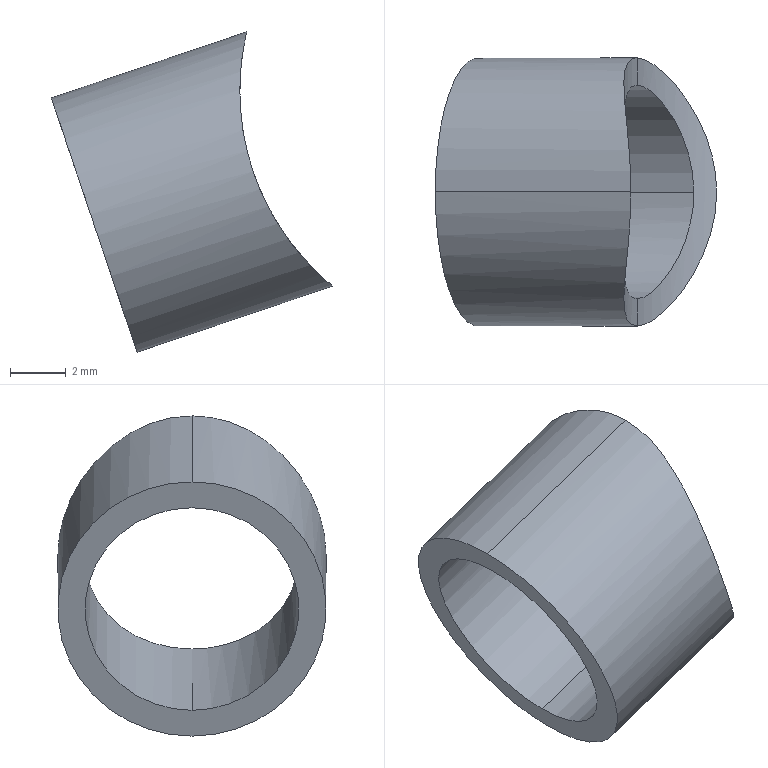Part | STEP file | 2026.6.15-Main Assembly图.sldasm-Part-265 | 1 solid | 7 faces | box 10.07 x 9.6 x 11.459 mm | volume 173.019 mm3 | cylinder 6 | plane 1 | commonest cylinder face diameters 7.65 x2 9.6 x2 18 x2
STEP:
#1=CARTESIAN_POINT('',(-1469.975,1419.464,3250.583));
#2=VERTEX_POINT('',#1);
#3=CARTESIAN_POINT('',(-1470.196,1424.264,3255.574));
#4=VERTEX_POINT('',#3);
#5=CARTESIAN_POINT('',(-1469.975,1419.464,3250.583));
#6=CARTESIAN_POINT('',(-1470.026,1419.464,3250.735));
#7=CARTESIAN_POINT('',(-1470.074,1419.472,3250.89));
#8=CARTESIAN_POINT('',(-1470.16,1419.505,3251.198));
#9=CARTESIAN_POINT('',(-1470.198,1419.529,3251.351));
#10=CARTESIAN_POINT('',(-1470.266,1419.592,3251.656));
#11=CARTESIAN_POINT('',(-1470.296,1419.631,3251.808));
#12=CARTESIAN_POINT('',(-1470.347,1419.724,3252.111));
#13=CARTESIAN_POINT('',(-1470.369,1419.779,3252.262));
#14=CARTESIAN_POINT('',(-1470.421,1419.963,3252.705));
#15=CARTESIAN_POINT('',(-1470.439,1420.111,3252.987));
#16=CARTESIAN_POINT('',(-1470.451,1420.459,3253.527));
#17=CARTESIAN_POINT('',(-1470.445,1420.658,3253.783));
#18=CARTESIAN_POINT('',(-1470.416,1421.092,3254.25));
#19=CARTESIAN_POINT('',(-1470.394,1421.33,3254.464));
#20=CARTESIAN_POINT('',(-1470.343,1421.847,3254.848));
#21=CARTESIAN_POINT('',(-1470.314,1422.118,3255.012));
#22=CARTESIAN_POINT('',(-1470.276,1422.548,3255.216));
#23=CARTESIAN_POINT('',(-1470.263,1422.695,3255.276));
#24=CARTESIAN_POINT('',(-1470.241,1422.996,3255.382));
#25=CARTESIAN_POINT('',(-1470.231,1423.152,3255.428));
#26=CARTESIAN_POINT('',(-1470.206,1423.622,3255.537));
#27=CARTESIAN_POINT('',(-1470.196,1423.94,3255.574));
#28=CARTESIAN_POINT('',(-1470.196,1424.264,3255.574));
#29=B_SPLINE_CURVE_WITH_KNOTS('',3,(#5,#6,#7,#8,#9,#10,#11,#12,#13,#14,#15,#16,#17,#18,#19,#20,#21,#22,#23,#24,#25,#26,#27,#28),.UNSPECIFIED.,.F.,.F.,(4,2,2,2,2,2,2,2,2,2,2,4),(0.007657,0.008135,0.008612,0.00909,0.009568,0.01052,0.01148,0.01243,0.01339,0.01387,0.01434,0.0153),.UNSPECIFIED.);
#30=EDGE_CURVE('',#2,#4,#29,.T.);
#31=ORIENTED_EDGE('',*,*,#30,.F.);
#32=CARTESIAN_POINT('',(-1469.975,1420.439,3250.583));
#33=VERTEX_POINT('',#32);
#34=CARTESIAN_POINT('',(-1469.975,1412.264,3250.583));
#35=DIRECTION('',(0.,1.,0.));
#36=VECTOR('',#35,1000.);
#37=LINE('',#34,#36);
#38=EDGE_CURVE('',#2,#33,#37,.T.);
#39=ORIENTED_EDGE('',*,*,#38,.T.);
#40=CARTESIAN_POINT('',(-1470.39,1424.264,3254.48));
#41=VERTEX_POINT('',#40);
#42=CARTESIAN_POINT('',(-1470.39,1424.264,3254.48));
#43=CARTESIAN_POINT('',(-1470.39,1424.008,3254.48));
#44=CARTESIAN_POINT('',(-1470.393,1423.757,3254.452));
#45=CARTESIAN_POINT('',(-1470.405,1423.264,3254.343));
#46=CARTESIAN_POINT('',(-1470.413,1423.02,3254.262));
#47=CARTESIAN_POINT('',(-1470.429,1422.558,3254.052));
#48=CARTESIAN_POINT('',(-1470.437,1422.34,3253.925));
#49=CARTESIAN_POINT('',(-1470.447,1421.926,3253.629));
#50=CARTESIAN_POINT('',(-1470.449,1421.733,3253.461));
#51=CARTESIAN_POINT('',(-1470.442,1421.385,3253.095));
#52=CARTESIAN_POINT('',(-1470.432,1421.227,3252.896));
#53=CARTESIAN_POINT('',(-1470.395,1420.948,3252.47));
#54=CARTESIAN_POINT('',(-1470.368,1420.831,3252.248));
#55=CARTESIAN_POINT('',(-1470.294,1420.639,3251.788));
#56=CARTESIAN_POINT('',(-1470.245,1420.564,3251.547));
#57=CARTESIAN_POINT('',(-1470.126,1420.464,3251.064));
#58=CARTESIAN_POINT('',(-1470.056,1420.439,3250.823));
#59=CARTESIAN_POINT('',(-1469.975,1420.439,3250.583));
#60=B_SPLINE_CURVE_WITH_KNOTS('',3,(#42,#43,#44,#45,#46,#47,#48,#49,#50,#51,#52,#53,#54,#55,#56,#57,#58,#59),.UNSPECIFIED.,.F.,.F.,(4,2,2,2,2,2,2,2,4),(0.,0.0007567,0.001513,0.00227,0.003027,0.003784,0.00454,0.005297,0.006054),.UNSPECIFIED.);
#61=EDGE_CURVE('',#41,#33,#60,.T.);
#62=ORIENTED_EDGE('',*,*,#61,.F.);
#63=CARTESIAN_POINT('',(-1469.975,1428.089,3250.583));
#64=VERTEX_POINT('',#63);
#65=CARTESIAN_POINT('',(-1469.975,1428.089,3250.583));
#66=CARTESIAN_POINT('',(-1470.055,1428.089,3250.822));
#67=CARTESIAN_POINT('',(-1470.127,1428.064,3251.069));
#68=CARTESIAN_POINT('',(-1470.245,1427.964,3251.549));
#69=CARTESIAN_POINT('',(-1470.293,1427.891,3251.787));
#70=CARTESIAN_POINT('',(-1470.369,1427.696,3252.253));
#71=CARTESIAN_POINT('',(-1470.396,1427.578,3252.474));
#72=CARTESIAN_POINT('',(-1470.432,1427.302,3252.896));
#73=CARTESIAN_POINT('',(-1470.442,1427.142,3253.098));
#74=CARTESIAN_POINT('',(-1470.449,1426.793,3253.463));
#75=CARTESIAN_POINT('',(-1470.447,1426.603,3253.629));
#76=CARTESIAN_POINT('',(-1470.437,1426.19,3253.925));
#77=CARTESIAN_POINT('',(-1470.429,1425.969,3254.053));
#78=CARTESIAN_POINT('',(-1470.413,1425.511,3254.261));
#79=CARTESIAN_POINT('',(-1470.405,1425.272,3254.341));
#80=CARTESIAN_POINT('',(-1470.393,1424.774,3254.452));
#81=CARTESIAN_POINT('',(-1470.39,1424.52,3254.48));
#82=CARTESIAN_POINT('',(-1470.39,1424.264,3254.48));
#83=B_SPLINE_CURVE_WITH_KNOTS('',3,(#65,#66,#67,#68,#69,#70,#71,#72,#73,#74,#75,#76,#77,#78,#79,#80,#81,#82),.UNSPECIFIED.,.F.,.F.,(4,2,2,2,2,2,2,2,4),(0.006054,0.006809,0.007565,0.00832,0.009076,0.009831,0.01059,0.01134,0.0121),.UNSPECIFIED.);
#84=EDGE_CURVE('',#64,#41,#83,.T.);
#85=ORIENTED_EDGE('',*,*,#84,.F.);
#86=CARTESIAN_POINT('',(-1469.975,1429.064,3250.583));
#87=VERTEX_POINT('',#86);
#88=CARTESIAN_POINT('',(-1469.975,1412.264,3250.583));
#89=DIRECTION('',(0.,1.,0.));
#90=VECTOR('',#89,1000.);
#91=LINE('',#88,#90);
#92=EDGE_CURVE('',#64,#87,#91,.T.);
#93=ORIENTED_EDGE('',*,*,#92,.T.);
#94=CARTESIAN_POINT('',(-1470.196,1424.264,3255.574));
#95=CARTESIAN_POINT('',(-1470.196,1424.589,3255.574));
#96=CARTESIAN_POINT('',(-1470.206,1424.906,3255.537));
#97=CARTESIAN_POINT('',(-1470.238,1425.528,3255.393));
#98=CARTESIAN_POINT('',(-1470.262,1425.835,3255.285));
#99=CARTESIAN_POINT('',(-1470.315,1426.412,3255.011));
#100=CARTESIAN_POINT('',(-1470.343,1426.685,3254.846));
#101=CARTESIAN_POINT('',(-1470.394,1427.202,3254.462));
#102=CARTESIAN_POINT('',(-1470.416,1427.44,3254.246));
#103=CARTESIAN_POINT('',(-1470.445,1427.875,3253.778));
#104=CARTESIAN_POINT('',(-1470.452,1428.074,3253.522));
#105=CARTESIAN_POINT('',(-1470.439,1428.421,3252.981));
#106=CARTESIAN_POINT('',(-1470.42,1428.568,3252.7));
#107=CARTESIAN_POINT('',(-1470.351,1428.811,3252.113));
#108=CARTESIAN_POINT('',(-1470.299,1428.906,3251.805));
#109=CARTESIAN_POINT('',(-1470.162,1429.032,3251.193));
#110=CARTESIAN_POINT('',(-1470.077,1429.064,3250.887));
#111=CARTESIAN_POINT('',(-1469.975,1429.064,3250.583));
#112=B_SPLINE_CURVE_WITH_KNOTS('',3,(#94,#95,#96,#97,#98,#99,#100,#101,#102,#103,#104,#105,#106,#107,#108,#109,#110,#111),.UNSPECIFIED.,.F.,.F.,(4,2,2,2,2,2,2,2,4),(0.,0.0009572,0.001914,0.002871,0.003829,0.004786,0.005743,0.0067,0.007657),.UNSPECIFIED.);
#113=EDGE_CURVE('',#4,#87,#112,.T.);
#114=ORIENTED_EDGE('',*,*,#113,.F.);
#115=EDGE_LOOP('',(#31,#39,#62,#85,#93,#114));
#116=FACE_OUTER_BOUND('',#115,.T.);
#117=CARTESIAN_POINT('',(-1461.448,1412.264,3253.462));
#118=DIRECTION('',(0.,1.,0.));
#119=DIRECTION('',(-0.9474,0.,-0.3199));
#120=AXIS2_PLACEMENT_3D('',#117,#118,#119);
#121=CYLINDRICAL_SURFACE('',#120,9.);
#122=ADVANCED_FACE('',(#116),#121,.F.);
#123=CARTESIAN_POINT('',(-1476.883,1424.264,3252.287));
#124=VERTEX_POINT('',#123);
#125=CARTESIAN_POINT('',(-1498.2,1424.264,3245.088));
#126=DIRECTION('',(0.9474,0.,0.3199));
#127=VECTOR('',#126,1000.);
#128=LINE('',#125,#127);
#129=EDGE_CURVE('',#124,#41,#128,.T.);
#130=ORIENTED_EDGE('',*,*,#129,.F.);
#131=CARTESIAN_POINT('',(-1474.435,1424.264,3245.039));
#132=VERTEX_POINT('',#131);
#133=CARTESIAN_POINT('',(-1475.659,1424.264,3248.663));
#134=DIRECTION('',(-0.9474,0.,-0.3199));
#135=DIRECTION('',(0.3199,0.,-0.9474));
#136=AXIS2_PLACEMENT_3D('',#133,#134,#135);
#137=CIRCLE('',#136,3.825);
#138=EDGE_CURVE('',#124,#132,#137,.T.);
#139=ORIENTED_EDGE('',*,*,#138,.T.);
#140=CARTESIAN_POINT('',(-1467.942,1424.264,3247.232));
#141=VERTEX_POINT('',#140);
#142=CARTESIAN_POINT('',(-1495.753,1424.264,3237.841));
#143=DIRECTION('',(0.9474,0.,0.3199));
#144=VECTOR('',#143,1000.);
#145=LINE('',#142,#144);
#146=EDGE_CURVE('',#132,#141,#145,.T.);
#147=ORIENTED_EDGE('',*,*,#146,.T.);
#148=CARTESIAN_POINT('',(-1467.942,1424.264,3247.232));
#149=CARTESIAN_POINT('',(-1467.942,1424.52,3247.232));
#150=CARTESIAN_POINT('',(-1467.962,1424.772,3247.252));
#151=CARTESIAN_POINT('',(-1468.037,1425.265,3247.332));
#152=CARTESIAN_POINT('',(-1468.093,1425.509,3247.392));
#153=CARTESIAN_POINT('',(-1468.233,1425.971,3247.548));
#154=CARTESIAN_POINT('',(-1468.316,1426.189,3247.644));
#155=CARTESIAN_POINT('',(-1468.504,1426.603,3247.874));
#156=CARTESIAN_POINT('',(-1468.608,1426.795,3248.007));
#157=CARTESIAN_POINT('',(-1468.823,1427.144,3248.302));
#158=CARTESIAN_POINT('',(-1468.936,1427.302,3248.466));
#159=CARTESIAN_POINT('',(-1469.165,1427.581,3248.827));
#160=CARTESIAN_POINT('',(-1469.278,1427.698,3249.02));
#161=CARTESIAN_POINT('',(-1469.498,1427.89,3249.431));
#162=CARTESIAN_POINT('',(-1469.605,1427.965,3249.653));
#163=CARTESIAN_POINT('',(-1469.803,1428.064,3250.109));
#164=CARTESIAN_POINT('',(-1469.894,1428.089,3250.343));
#165=CARTESIAN_POINT('',(-1469.975,1428.089,3250.583));
#166=B_SPLINE_CURVE_WITH_KNOTS('',3,(#148,#149,#150,#151,#152,#153,#154,#155,#156,#157,#158,#159,#160,#161,#162,#163,#164,#165),.UNSPECIFIED.,.F.,.F.,(4,2,2,2,2,2,2,2,4),(0.,0.0007567,0.001513,0.00227,0.003027,0.003784,0.00454,0.005297,0.006054),.UNSPECIFIED.);
#167=EDGE_CURVE('',#141,#64,#166,.T.);
#168=ORIENTED_EDGE('',*,*,#167,.T.);
#169=ORIENTED_EDGE('',*,*,#84,.T.);
#170=EDGE_LOOP('',(#130,#139,#147,#168,#169));
#171=FACE_OUTER_BOUND('',#170,.T.);
#172=CARTESIAN_POINT('',(-1496.977,1424.264,3241.465));
#173=DIRECTION('',(0.9474,0.,0.3199));
#174=DIRECTION('',(-0.3199,0.,0.9474));
#175=AXIS2_PLACEMENT_3D('',#172,#173,#174);
#176=CYLINDRICAL_SURFACE('',#175,3.825);
#177=ADVANCED_FACE('',(#171),#176,.F.);
#178=CARTESIAN_POINT('',(-1474.123,1424.264,3244.116));
#179=VERTEX_POINT('',#178);
#180=CARTESIAN_POINT('',(-1477.195,1424.264,3253.211));
#181=VERTEX_POINT('',#180);
#182=CARTESIAN_POINT('',(-1475.659,1424.264,3248.663));
#183=DIRECTION('',(0.9474,0.,0.3199));
#184=DIRECTION('',(0.3199,0.,-0.9474));
#185=AXIS2_PLACEMENT_3D('',#182,#183,#184);
#186=CIRCLE('',#185,4.8);
#187=EDGE_CURVE('',#179,#181,#186,.T.);
#188=ORIENTED_EDGE('',*,*,#187,.F.);
#189=CARTESIAN_POINT('',(-1475.659,1424.264,3248.663));
#190=DIRECTION('',(0.9474,0.,0.3199));
#191=DIRECTION('',(0.3199,0.,-0.9474));
#192=AXIS2_PLACEMENT_3D('',#189,#190,#191);
#193=CIRCLE('',#192,4.8);
#194=EDGE_CURVE('',#181,#179,#193,.T.);
#195=ORIENTED_EDGE('',*,*,#194,.F.);
#196=EDGE_LOOP('',(#188,#195));
#197=FACE_OUTER_BOUND('',#196,.T.);
#198=CARTESIAN_POINT('',(-1475.659,1424.264,3248.663));
#199=DIRECTION('',(-0.9474,0.,-0.3199));
#200=DIRECTION('',(0.3199,0.,-0.9474));
#201=AXIS2_PLACEMENT_3D('',#198,#199,#200);
#202=CIRCLE('',#201,3.825);
#203=EDGE_CURVE('',#132,#124,#202,.T.);
#204=ORIENTED_EDGE('',*,*,#203,.F.);
#205=ORIENTED_EDGE('',*,*,#138,.F.);
#206=EDGE_LOOP('',(#204,#205));
#207=FACE_BOUND('',#206,.T.);
#208=CARTESIAN_POINT('',(-1475.659,1424.264,3248.663));
#209=DIRECTION('',(0.9474,0.,0.3199));
#210=DIRECTION('',(-0.3199,0.,0.9474));
#211=AXIS2_PLACEMENT_3D('',#208,#209,#210);
#212=PLANE('',#211);
#213=ADVANCED_FACE('',(#197,#207),#212,.F.);
#214=ORIENTED_EDGE('',*,*,#38,.F.);
#215=CARTESIAN_POINT('',(-1467.125,1424.264,3246.479));
#216=VERTEX_POINT('',#215);
#217=CARTESIAN_POINT('',(-1467.125,1424.264,3246.479));
#218=CARTESIAN_POINT('',(-1467.125,1423.94,3246.479));
#219=CARTESIAN_POINT('',(-1467.155,1423.623,3246.503));
#220=CARTESIAN_POINT('',(-1467.268,1423.001,3246.598));
#221=CARTESIAN_POINT('',(-1467.353,1422.694,3246.669));
#222=CARTESIAN_POINT('',(-1467.56,1422.116,3246.855));
#223=CARTESIAN_POINT('',(-1467.683,1421.844,3246.97));
#224=CARTESIAN_POINT('',(-1467.957,1421.327,3247.244));
#225=CARTESIAN_POINT('',(-1468.105,1421.089,3247.402));
#226=CARTESIAN_POINT('',(-1468.412,1420.654,3247.756));
#227=CARTESIAN_POINT('',(-1468.572,1420.455,3247.957));
#228=CARTESIAN_POINT('',(-1468.89,1420.108,3248.394));
#229=CARTESIAN_POINT('',(-1469.046,1419.96,3248.63));
#230=CARTESIAN_POINT('',(-1469.346,1419.718,3249.138));
#231=CARTESIAN_POINT('',(-1469.492,1419.622,3249.414));
#232=CARTESIAN_POINT('',(-1469.754,1419.496,3249.984));
#233=CARTESIAN_POINT('',(-1469.872,1419.464,3250.279));
#234=CARTESIAN_POINT('',(-1469.975,1419.464,3250.583));
#235=B_SPLINE_CURVE_WITH_KNOTS('',3,(#217,#218,#219,#220,#221,#222,#223,#224,#225,#226,#227,#228,#229,#230,#231,#232,#233,#234),.UNSPECIFIED.,.F.,.F.,(4,2,2,2,2,2,2,2,4),(0.,0.0009572,0.001914,0.002871,0.003829,0.004786,0.005743,0.0067,0.007657),.UNSPECIFIED.);
#236=EDGE_CURVE('',#216,#2,#235,.T.);
#237=ORIENTED_EDGE('',*,*,#236,.F.);
#238=CARTESIAN_POINT('',(-1469.975,1429.064,3250.583));
#239=CARTESIAN_POINT('',(-1469.923,1429.064,3250.431));
#240=CARTESIAN_POINT('',(-1469.867,1429.056,3250.279));
#241=CARTESIAN_POINT('',(-1469.749,1429.024,3249.982));
#242=CARTESIAN_POINT('',(-1469.686,1429.,3249.837));
#243=CARTESIAN_POINT('',(-1469.556,1428.937,3249.553));
#244=CARTESIAN_POINT('',(-1469.487,1428.898,3249.414));
#245=CARTESIAN_POINT('',(-1469.344,1428.804,3249.142));
#246=CARTESIAN_POINT('',(-1469.27,1428.749,3249.009));
#247=CARTESIAN_POINT('',(-1469.043,1428.566,3248.625));
#248=CARTESIAN_POINT('',(-1468.886,1428.417,3248.389));
#249=CARTESIAN_POINT('',(-1468.569,1428.07,3247.953));
#250=CARTESIAN_POINT('',(-1468.409,1427.871,3247.753));
#251=CARTESIAN_POINT('',(-1468.103,1427.436,3247.399));
#252=CARTESIAN_POINT('',(-1467.955,1427.199,3247.242));
#253=CARTESIAN_POINT('',(-1467.682,1426.682,3246.968));
#254=CARTESIAN_POINT('',(-1467.56,1426.41,3246.855));
#255=CARTESIAN_POINT('',(-1467.405,1425.981,3246.716));
#256=CARTESIAN_POINT('',(-1467.359,1425.834,3246.676));
#257=CARTESIAN_POINT('',(-1467.277,1425.532,3246.605));
#258=CARTESIAN_POINT('',(-1467.241,1425.377,3246.575));
#259=CARTESIAN_POINT('',(-1467.155,1424.907,3246.503));
#260=CARTESIAN_POINT('',(-1467.125,1424.588,3246.479));
#261=CARTESIAN_POINT('',(-1467.125,1424.264,3246.479));
#262=B_SPLINE_CURVE_WITH_KNOTS('',3,(#238,#239,#240,#241,#242,#243,#244,#245,#246,#247,#248,#249,#250,#251,#252,#253,#254,#255,#256,#257,#258,#259,#260,#261),.UNSPECIFIED.,.F.,.F.,(4,2,2,2,2,2,2,2,2,2,2,4),(0.007657,0.008135,0.008612,0.00909,0.009568,0.01052,0.01148,0.01243,0.01339,0.01387,0.01434,0.0153),.UNSPECIFIED.);
#263=EDGE_CURVE('',#87,#216,#262,.T.);
#264=ORIENTED_EDGE('',*,*,#263,.F.);
#265=ORIENTED_EDGE('',*,*,#92,.F.);
#266=ORIENTED_EDGE('',*,*,#167,.F.);
#267=CARTESIAN_POINT('',(-1469.975,1420.439,3250.583));
#268=CARTESIAN_POINT('',(-1469.894,1420.439,3250.343));
#269=CARTESIAN_POINT('',(-1469.801,1420.465,3250.104));
#270=CARTESIAN_POINT('',(-1469.604,1420.564,3249.65));
#271=CARTESIAN_POINT('',(-1469.498,1420.638,3249.432));
#272=CARTESIAN_POINT('',(-1469.276,1420.833,3249.016));
#273=CARTESIAN_POINT('',(-1469.163,1420.951,3248.823));
#274=CARTESIAN_POINT('',(-1468.936,1421.227,3248.466));
#275=CARTESIAN_POINT('',(-1468.822,1421.387,3248.3));
#276=CARTESIAN_POINT('',(-1468.606,1421.736,3248.004));
#277=CARTESIAN_POINT('',(-1468.504,1421.926,3247.874));
#278=CARTESIAN_POINT('',(-1468.316,1422.338,3247.645));
#279=CARTESIAN_POINT('',(-1468.232,1422.56,3247.548));
#280=CARTESIAN_POINT('',(-1468.093,1423.018,3247.392));
#281=CARTESIAN_POINT('',(-1468.038,1423.256,3247.333));
#282=CARTESIAN_POINT('',(-1467.962,1423.755,3247.252));
#283=CARTESIAN_POINT('',(-1467.942,1424.008,3247.232));
#284=CARTESIAN_POINT('',(-1467.942,1424.264,3247.232));
#285=B_SPLINE_CURVE_WITH_KNOTS('',3,(#267,#268,#269,#270,#271,#272,#273,#274,#275,#276,#277,#278,#279,#280,#281,#282,#283,#284),.UNSPECIFIED.,.F.,.F.,(4,2,2,2,2,2,2,2,4),(0.006054,0.006809,0.007565,0.00832,0.009076,0.009831,0.01059,0.01134,0.0121),.UNSPECIFIED.);
#286=EDGE_CURVE('',#33,#141,#285,.T.);
#287=ORIENTED_EDGE('',*,*,#286,.F.);
#288=EDGE_LOOP('',(#214,#237,#264,#265,#266,#287));
#289=FACE_OUTER_BOUND('',#288,.T.);
#290=CARTESIAN_POINT('',(-1461.448,1412.264,3253.462));
#291=DIRECTION('',(0.,1.,0.));
#292=DIRECTION('',(-0.9474,0.,-0.3199));
#293=AXIS2_PLACEMENT_3D('',#290,#291,#292);
#294=CYLINDRICAL_SURFACE('',#293,9.);
#295=ADVANCED_FACE('',(#289),#294,.F.);
#296=CARTESIAN_POINT('',(-1462.983,1424.264,3258.01));
#297=DIRECTION('',(0.9474,0.,0.3199));
#298=VECTOR('',#297,1000.);
#299=LINE('',#296,#298);
#300=EDGE_CURVE('',#181,#4,#299,.T.);
#301=ORIENTED_EDGE('',*,*,#300,.F.);
#302=ORIENTED_EDGE('',*,*,#194,.T.);
#303=CARTESIAN_POINT('',(-1459.912,1424.264,3248.915));
#304=DIRECTION('',(0.9474,0.,0.3199));
#305=VECTOR('',#304,1000.);
#306=LINE('',#303,#305);
#307=EDGE_CURVE('',#179,#216,#306,.T.);
#308=ORIENTED_EDGE('',*,*,#307,.T.);
#309=ORIENTED_EDGE('',*,*,#236,.T.);
#310=ORIENTED_EDGE('',*,*,#30,.T.);
#311=EDGE_LOOP('',(#301,#302,#308,#309,#310));
#312=FACE_OUTER_BOUND('',#311,.T.);
#313=CARTESIAN_POINT('',(-1461.448,1424.264,3253.462));
#314=DIRECTION('',(0.9474,0.,0.3199));
#315=DIRECTION('',(-0.3199,0.,0.9474));
#316=AXIS2_PLACEMENT_3D('',#313,#314,#315);
#317=CYLINDRICAL_SURFACE('',#316,4.8);
#318=ADVANCED_FACE('',(#312),#317,.T.);
#319=ORIENTED_EDGE('',*,*,#203,.T.);
#320=ORIENTED_EDGE('',*,*,#129,.T.);
#321=ORIENTED_EDGE('',*,*,#61,.T.);
#322=ORIENTED_EDGE('',*,*,#286,.T.);
#323=ORIENTED_EDGE('',*,*,#146,.F.);
#324=EDGE_LOOP('',(#319,#320,#321,#322,#323));
#325=FACE_OUTER_BOUND('',#324,.T.);
#326=CARTESIAN_POINT('',(-1496.977,1424.264,3241.465));
#327=DIRECTION('',(0.9474,0.,0.3199));
#328=DIRECTION('',(-0.3199,0.,0.9474));
#329=AXIS2_PLACEMENT_3D('',#326,#327,#328);
#330=CYLINDRICAL_SURFACE('',#329,3.825);
#331=ADVANCED_FACE('',(#325),#330,.F.);
#332=ORIENTED_EDGE('',*,*,#187,.T.);
#333=ORIENTED_EDGE('',*,*,#300,.T.);
#334=ORIENTED_EDGE('',*,*,#113,.T.);
#335=ORIENTED_EDGE('',*,*,#263,.T.);
#336=ORIENTED_EDGE('',*,*,#307,.F.);
#337=EDGE_LOOP('',(#332,#333,#334,#335,#336));
#338=FACE_OUTER_BOUND('',#337,.T.);
#339=CARTESIAN_POINT('',(-1461.448,1424.264,3253.462));
#340=DIRECTION('',(0.9474,0.,0.3199));
#341=DIRECTION('',(-0.3199,0.,0.9474));
#342=AXIS2_PLACEMENT_3D('',#339,#340,#341);
#343=CYLINDRICAL_SURFACE('',#342,4.8);
#344=ADVANCED_FACE('',(#338),#343,.T.);
#345=CLOSED_SHELL('',(#122,#177,#213,#295,#318,#331,#344));
#346=MANIFOLD_SOLID_BREP('',#345);
#347=CARTESIAN_POINT('',(0.,0.,0.));
#348=DIRECTION('',(0.,0.,1.));
#349=DIRECTION('',(1.,0.,0.));
#350=AXIS2_PLACEMENT_3D('',#347,#348,#349);
#351=(LENGTH_UNIT()NAMED_UNIT(*)SI_UNIT(.MILLI.,.METRE.));
#352=UNCERTAINTY_MEASURE_WITH_UNIT(LENGTH_MEASURE(0.00001),#351,'','');
#353=(NAMED_UNIT(*)PLANE_ANGLE_UNIT()SI_UNIT($,.RADIAN.));
#354=(NAMED_UNIT(*)SI_UNIT($,.STERADIAN.)SOLID_ANGLE_UNIT());
#355=(GEOMETRIC_REPRESENTATION_CONTEXT(3)GLOBAL_UNCERTAINTY_ASSIGNED_CONTEXT((#352))GLOBAL_UNIT_ASSIGNED_CONTEXT((#351,#353,#354))REPRESENTATION_CONTEXT('',''));
#356=ADVANCED_BREP_SHAPE_REPRESENTATION('',(#346,#350),#355);